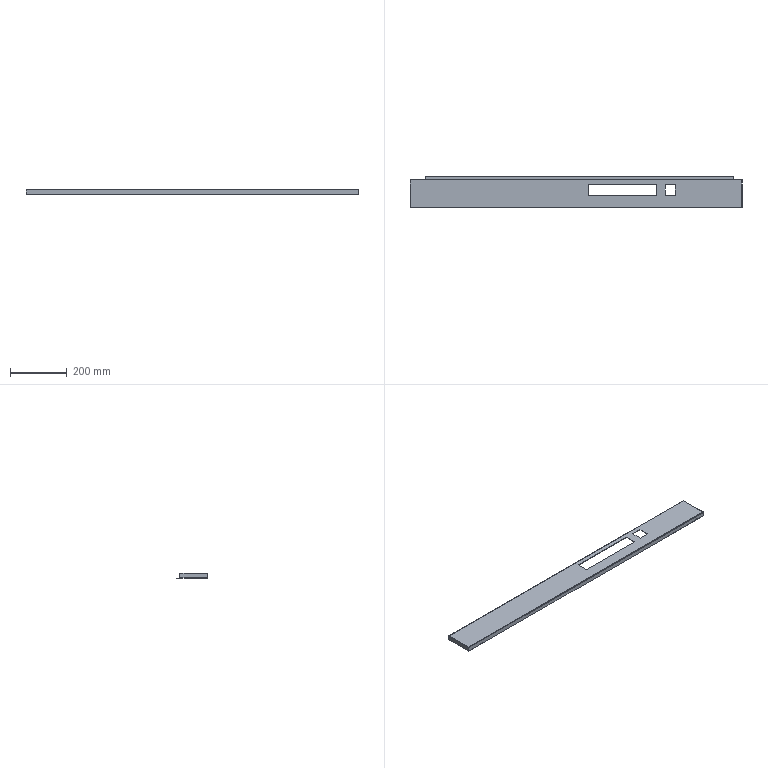Part | NX | features BREP 3 | 3 solids | 98 faces | box 1169 x 112 x 18 mm | volume 246191 mm3 | plane 80 | cylinder 18 | commonest cylinder face diameters 0.02 x7 3.02 x7 3.3 x4